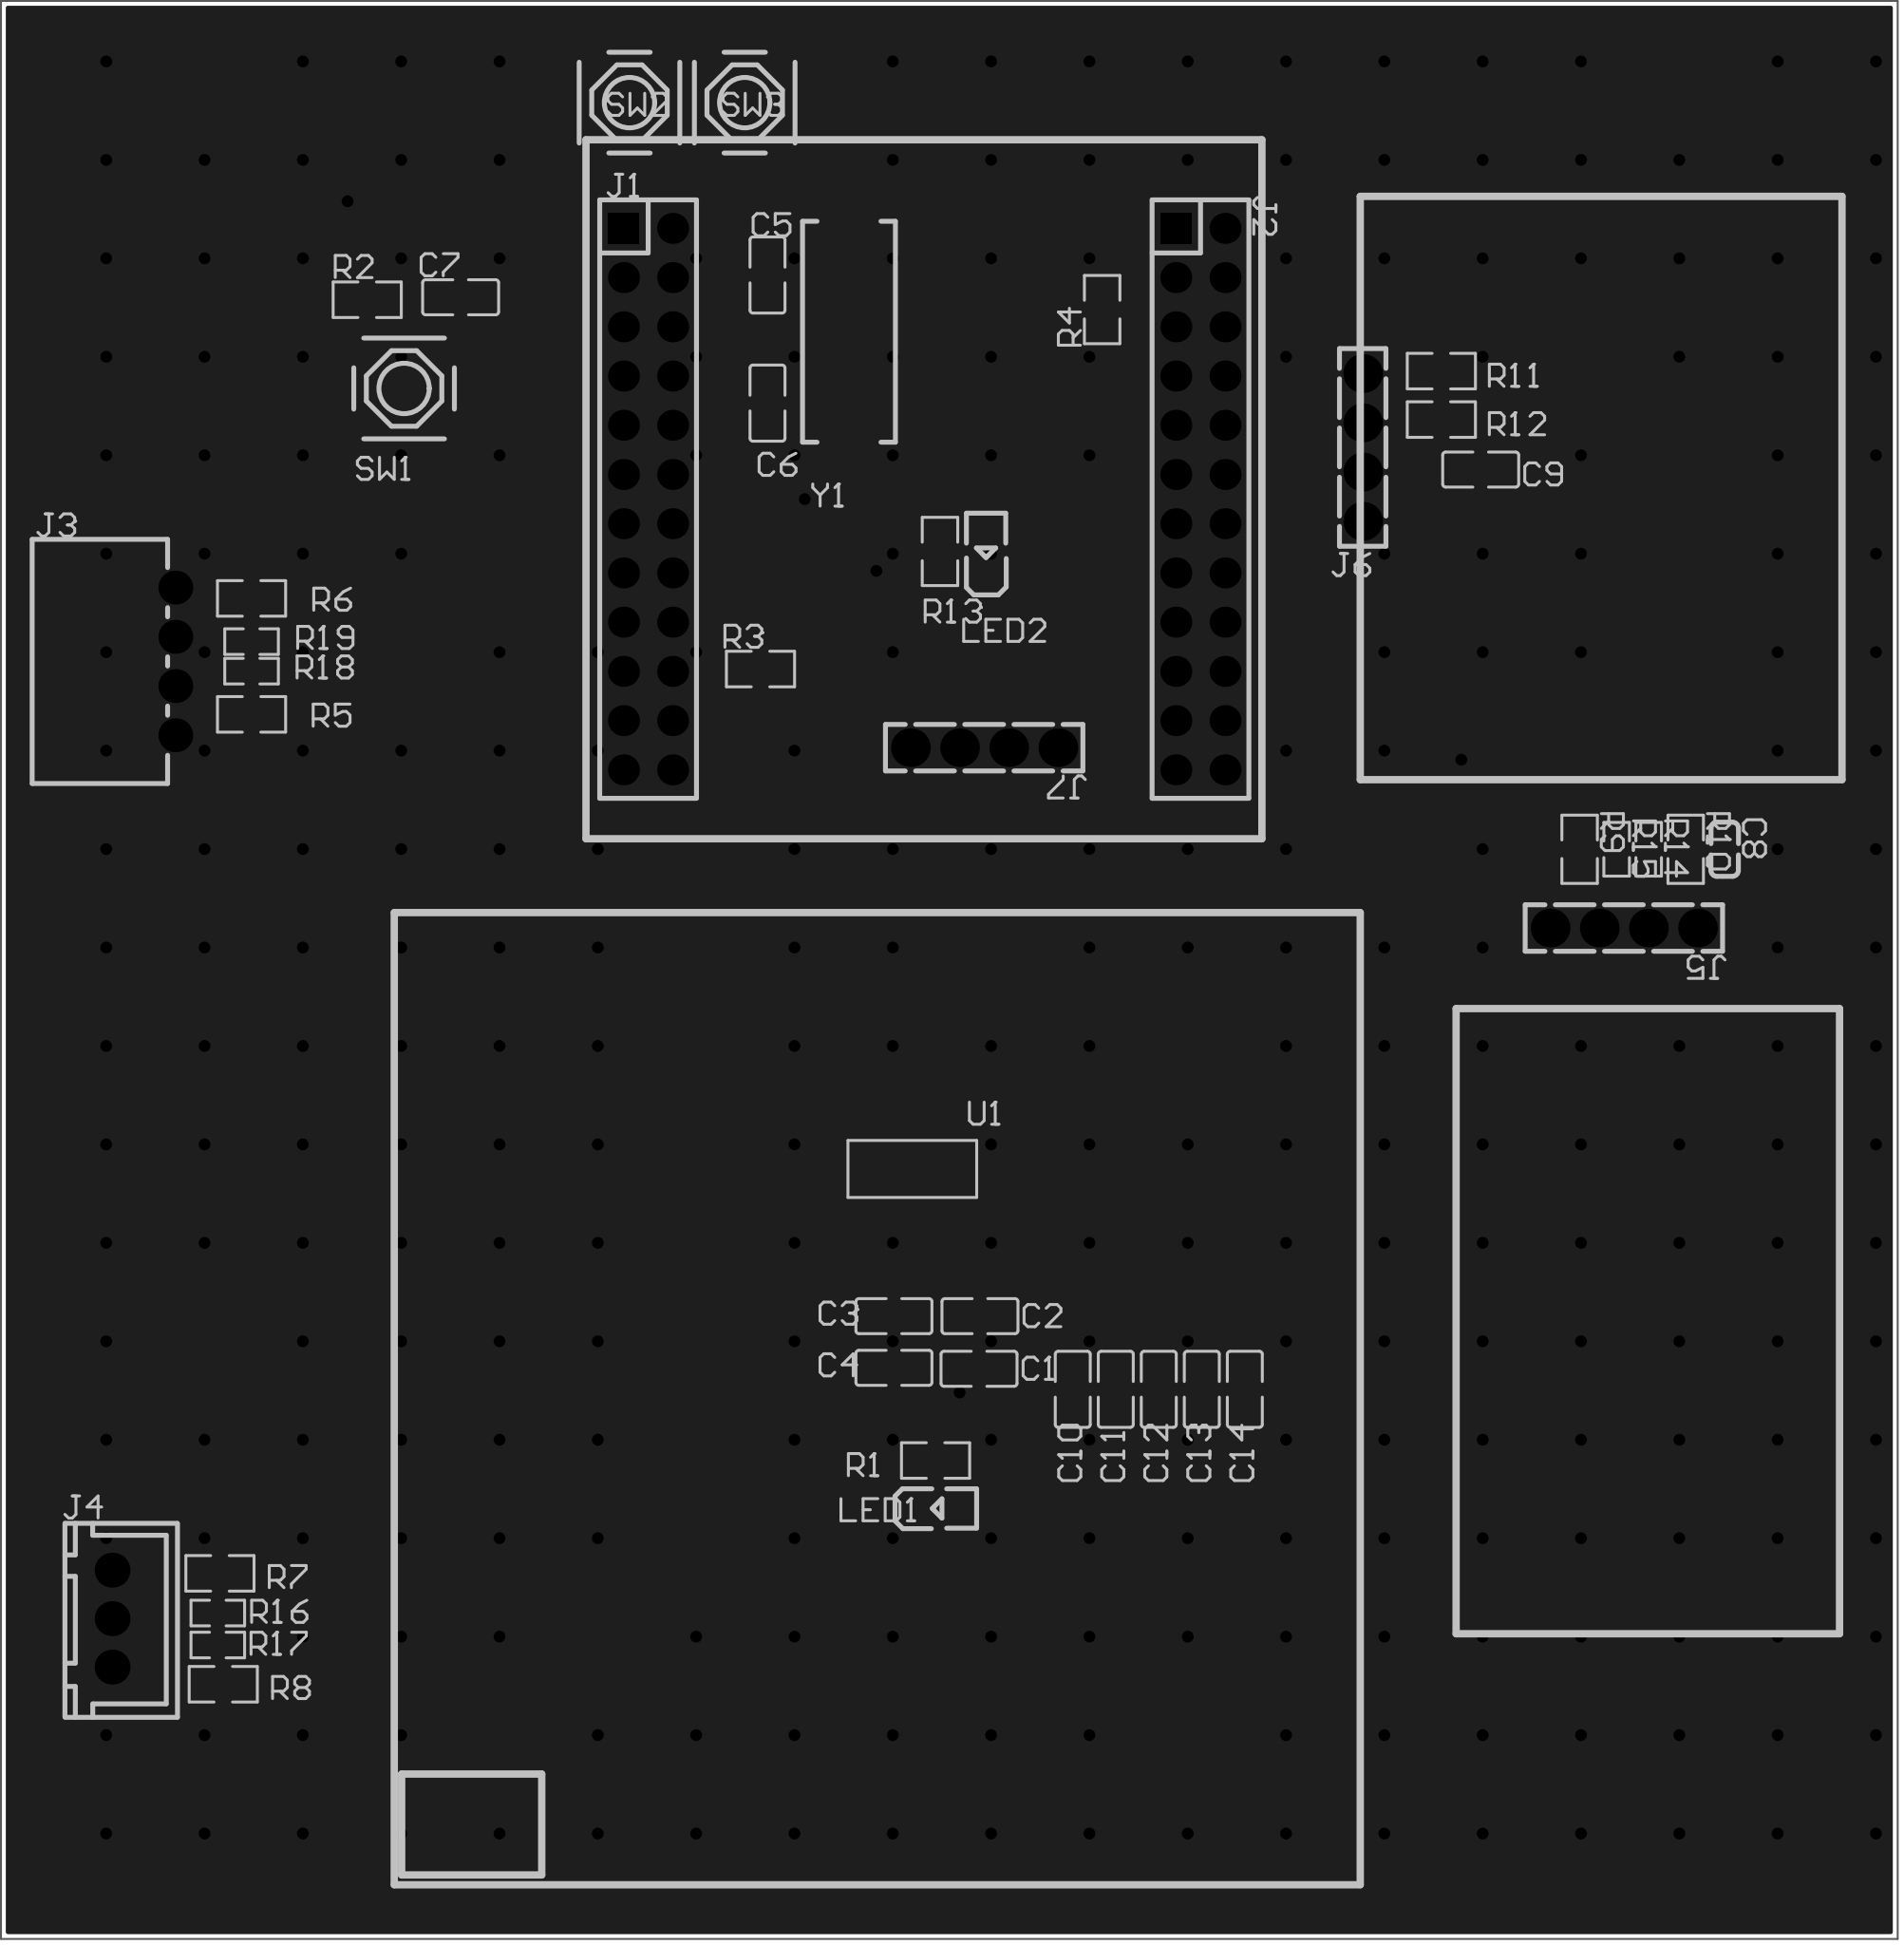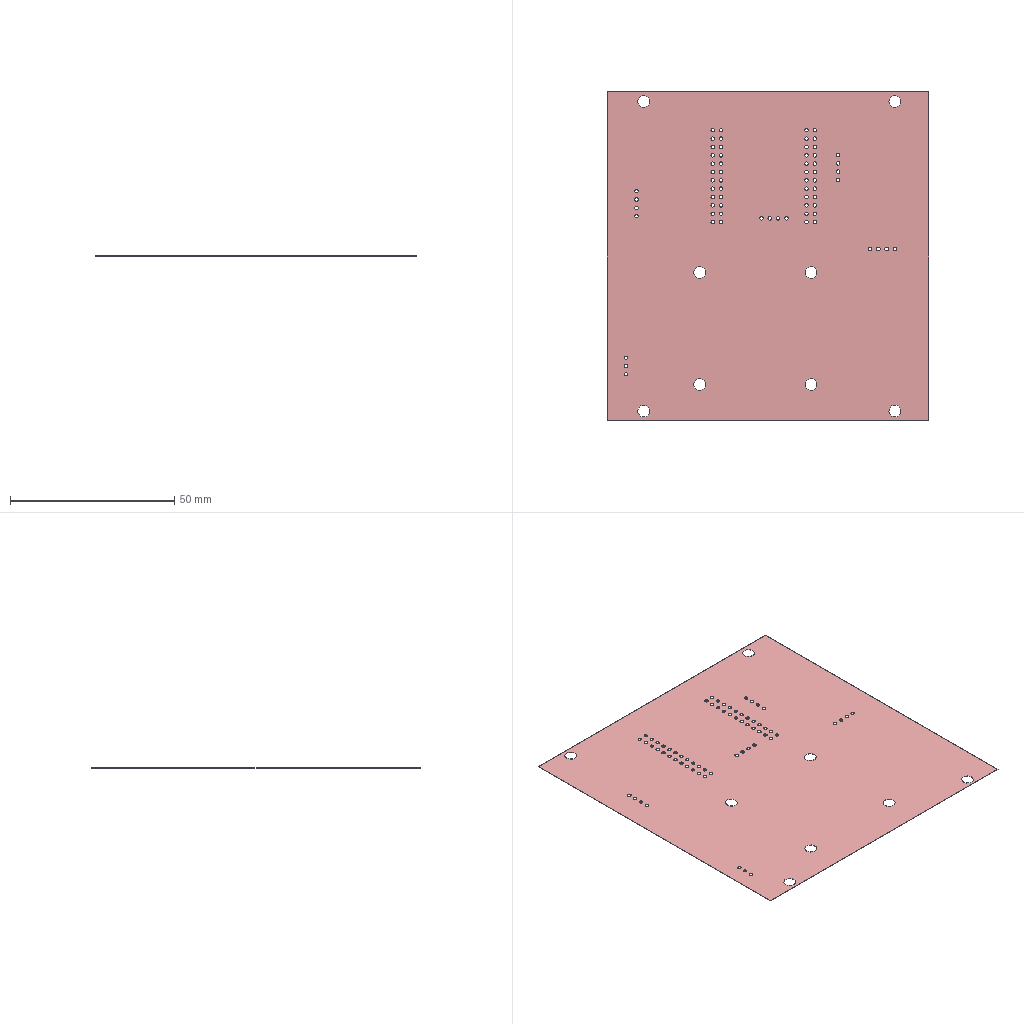Circuit board layout | Altium Designer | box 98 x 100 x 0.1 mm
Layer stack:
# Altium Designer layer stack of  (unit mm; dielectric type: 0 none, 1 core, 2 prepreg, 3 surface material)
index,name,kind,layer,copper_thickness_mm,dielectric_type,dielectric_thickness_mm,dielectric_material,dielectric_constant
0,Top Paste Mask Layer,other,,,,,,
1,Top Silkscreen Layer,other,,,,,,
2,Top Solder Mask Layer,dielectric,,,3,0.01,,3.3
3,Top Layer,copper,Top Layer,0.035,,,,
4,Bottom Layer,copper,Bottom Layer,0.035,,,,
5,Bottom Solder Mask Layer,dielectric,,,3,0.01,,3.3
6,Bottom Silkscreen Layer,other,,,,,,
7,Bottom Paste Mask Layer,other,,,,,,
# drill layer pairs: low layer,high layer
drill_pair,Top Layer,Bottom Layer
Part placement:
Designator,Comment,Layer,Footprint,Center-X(mm),Center-Y(mm),Rotation
C1,10uF,TopLayer,C0805,147.054,125.178,0
C2,0.1uF,TopLayer,C0805,147.102,127.894,0
C3,10uF,TopLayer,C0805,142.657,127.894,0
C4,0.1uF,TopLayer,C0805,142.657,125.227,0
C5,20pF,TopLayer,C0805,136.125,181.616,270
C6,20pF,TopLayer,C0805,136.125,175.006,90
C7,10uF,TopLayer,C0805,120.269,180.467,0
C9,0.1uF,TopLayer,C0805,172.974,171.577,0
C10,0.1uF,TopLayer,C0805,151.897,124.118,90
C11,0.1uF,TopLayer,C0805,154.12,124.118,90
C12,0.1uF,TopLayer,C0805,156.342,124.118,90
C13,0.1uF,TopLayer,C0805,158.565,124.118,90
C14,0.1uF,TopLayer,C0805,160.787,124.118,90
J6,,TopLayer,CONN-TH_4P-P2.54-L10.2-W2.5,166.878,172.72,90
J7,,TopLayer,CONN-TH_4P-P2.54-L10.2-W2.5,147.32,157.226,180
LED1,KT-0805W,TopLayer,LED0805-R-RD,144.938,117.971,0
LED2,,TopLayer,LED0805-R-RD,147.418,167.334,90
R1,510,TopLayer,R0805,144.809,120.445,0
R2,10K,TopLayer,R0805,115.443,180.34,180
R3,10K,TopLayer,R0805,135.763,161.284,0
R4,10K,TopLayer,R0805,153.416,179.832,90
R11,4.7K,TopLayer,R0805,170.942,176.657,0
R12,4.7K,TopLayer,R0805,170.942,174.157,0
R13,510,TopLayer,R0805,145.037,167.352,90
SW1,TS-1087S,TopLayer,SW-SMD_L5.2-W5.2-P3.70-LS6.4,117.348,175.762,0
SW2,TS-1087S,TopLayer,SW-SMD_L5.2-W5.2-P3.70-LS6.4,128.994,190.51,90
SW3,TS-1087S,TopLayer,SW-SMD_L5.2-W5.2-P3.70-LS6.4,134.948,190.51,90
U1,AMS1117-3.3,TopLayer,SOT-223-3_L6.5-W3.4-P2.30-LS7.0-BR,143.608,135.389,270
Y1,8MHz,TopLayer,CRYSTAL-SMD_L11.5-W4.8-LS12.7,140.335,178.689,90
C8,0.1uF,TopLayer,C0603,185.579,151.977,270
J1,PM254-2-12-Z-8.5,TopLayer,HDR-TH_24P-P2.54-V-F-R2-C12-S2.54-2,129.956,170.053,270
J2,PM254-2-12-Z-8.5,TopLayer,HDR-TH_24P-P2.54-V-F-R2-C12-S2.54-2,158.496,170.053,270
J3,XH-4AW,TopLayer,CONN-TH_XH-4AW,105.53,161.677,270
J4,XH-3A,TopLayer,CONN-TH_XH-3A,102.262,112.285,270
J5,,TopLayer,CONN-TH_4P-P2.54-L10.2-W2.5,180.372,147.921,180
R5,22R,TopLayer,R0805,109.467,158.945,180
R6,22R,TopLayer,R0805,109.467,164.929,180
R7,22R,TopLayer,R0805,107.834,114.623,180
R8,22R,TopLayer,R0805,108.005,108.9,180
R9,22R,TopLayer,R0805,178.086,151.985,270
R10,22R,TopLayer,R0805,183.567,151.985,270
R14,0R,TopLayer,R0603,181.654,151.985,270
R15,0R,TopLayer,R0603,179.998,151.985,270
R16,0R,TopLayer,R0603,107.723,112.575,180
R17,0R,TopLayer,R0603,107.723,110.924,180
R18,0R,TopLayer,R0603,109.467,161.175,180
R19,0R,TopLayer,R0603,109.467,162.699,180
Pad and via stacks:
# Altium Designer via and pad stacks of  (unit mm). Each distinct definition once, with the count of objects using it.
# via: kind,start_layer,end_layer,hole_mm,diameter_mm,mode(0 simple;1 top-mid-bottom;2 full stack),diameter_per_layer,count,example_net
# pad: kind,layer,hole_mm,hole_type(0 round;1 square;2 slot),plating,top_size,top_shape(1 round;2 rect;3 octagon;9 rounded rect),mid_size,bottom_size,mode,footprint,size_per_layer,count,example
pad,Top Layer,0,0,plated,1.41x1.35,2,1.41x1.35,1.41x1.35,0,C0805,,26,C1.2
pad,Top Layer,0,0,plated,1x1.399,2,1x1.399,1x1.399,0,LED0805-R-RD,,4,LED1.2
pad,Top Layer,0,0,plated,1.133x1.377,2,1.133x1.377,1.133x1.377,0,R0805,,26,R1.2
pad,Top Layer,0,0,plated,1.8x1.1,2,1.8x1.1,1.8x1.1,0,SW-SMD_L5.2-W5.2-P3.70-LS6.4,,12,SW1.1
pad,Top Layer,0,0,plated,2.5x1.1,2,2.5x1.1,2.5x1.1,0,SOT-223-3_L6.5-W3.4-P2.30-LS7.0-BR,,3,U1.1
pad,Top Layer,0,0,plated,2.34x3.6,2,2.34x3.6,2.34x3.6,0,SOT-223-3_L6.5-W3.4-P2.30-LS7.0-BR,,1,U1.4
pad,Top Layer,0,0,plated,5.5x2,2,5.5x2,5.5x2,0,CRYSTAL-SMD_L11.5-W4.8-LS12.7,,2,Y1.2
pad,Top Layer,0,0,plated,0.8x0.9,2,0.8x0.9,0.8x0.9,0,C0603,,2,C8.2
pad,Top Layer,0,0,plated,0.8065x0.864,2,0.8065x0.864,0.8065x0.864,0,R0603,,12,R14.2
pad,Multi-Layer,1.1,0,plated,2x2,1,2x2,2x2,0,CONN-TH_4P-P2.54-L10.2-W2.5,,12,J6.1
pad,Multi-Layer,1.05,0,plated,1.6x1.6,1,1.6x1.6,1.6x1.6,0,HDR-TH_24P-P2.54-V-F-R2-C12-S2.54-2,,46,J1.24
pad,Multi-Layer,1.05,0,plated,1.6x1.6,2,1.6x1.6,1.6x1.6,0,HDR-TH_24P-P2.54-V-F-R2-C12-S2.54-2,,2,J1.1
pad,Multi-Layer,1.1,0,plated,1.75x1.75,1,1.75x1.75,1.75x1.75,0,CONN-TH_XH-4AW,,4,J3.1
pad,Multi-Layer,1,0,plated,1.8x1.8,1,1.8x1.8,1.8x1.8,0,CONN-TH_XH-3A,,3,J4.1
via,Top Layer,Bottom Layer,0.3048,0.61,0,,300,PA1
Copper pours:
name,layer,net,type(0 solid;1 hatched;2 none)
Top Layer-GND,Top Layer,GND,0
Bottom Layer-GND,Bottom Layer,GND,0
Design rules, without the lines most boards share:
# Altium Designer design rules of  (exported by Altium Designer, unit mm)
# columns: name | kind | enabled | priority | scope1 | scope2 | descriptor | typed fields (field=value)
Plane_innerPlane | 0 | disabled | 1 | All | All | Clearance Constraint (Gap=6mil) (Disabled)(All),(All) | gap=0.1524
Plane_innerPlane_1 | 63 | disabled | 1 | All | All | Board Clearance Constraint (Gap=0mil) (Disabled)(All) |
Copper_copperRegion | 0 | disabled | 2 | All | All | Clearance Constraint (Gap=6mil) (Disabled)(All),(All) | gap=0.1524
Copper_copperRegion_1 | 63 | disabled | 2 | All | All | Board Clearance Constraint (Gap=0mil) (Disabled)(All) |
copperThickness1oz | 0 | enabled | 3 | All | All | Clearance Constraint (Gap=6mil) (All),(All) | gap=0.1524
copperThickness1oz_1 | 63 | enabled | 3 | All | All | Board Clearance Constraint (Gap=0mil) (All) |
otherClearance | 52 | enabled | 1 | All | All | Hole To Hole Clearance (Gap=11.8mil) (All),(All) | gap=0.2997
copperThickness1oz_2 | 2 | enabled | 1 | All | All | Width Constraint (Min=5mil) (Max=100mil) (Preferred=10mil) (All) |
differentialPair | 51 | enabled | 1 | All | All | Differential Pairs Uncoupled Length using the Gap Constraints (Min=5mil) (Max=6mil) (Prefered=6mil)  and Width Constraints (Min=5mil) (Max=100mil) (Prefered=100mil) (All) |
viaSize | 11 | enabled | 1 | All | All | Routing Via (MinHoleWidth=11.811mil) (MaxHoleWidth=248.032mil) (PreferredHoleWidth=12.008mil) (MinWidth=19.685mil) (MaxWidth=393.701mil) (PreferedWidth=24.016mil) (All) | via_min_hole=0.3 via_max_hole=6.3 via_preferred_diameter=0.61 via_preferred_hole=0.305